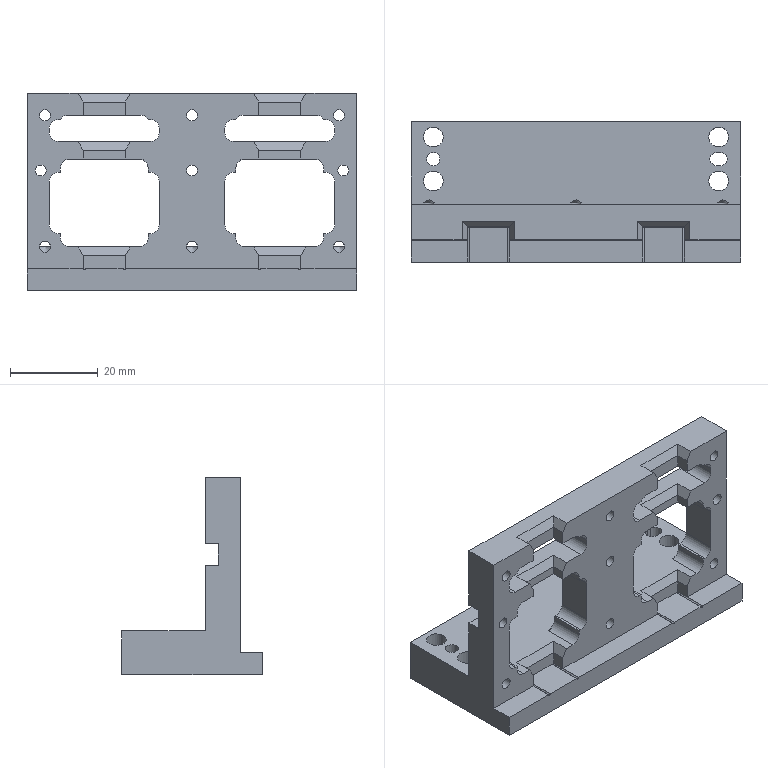Part | 1 solid | 151 faces | box 75 x 32 x 45 mm | volume 30935 mm3 | plane 100 | cylinder 48 | cone 3 | commonest cylinder face diameters 4 x28 2.5 x9 0.5 x4 4.5 x4 3 x3